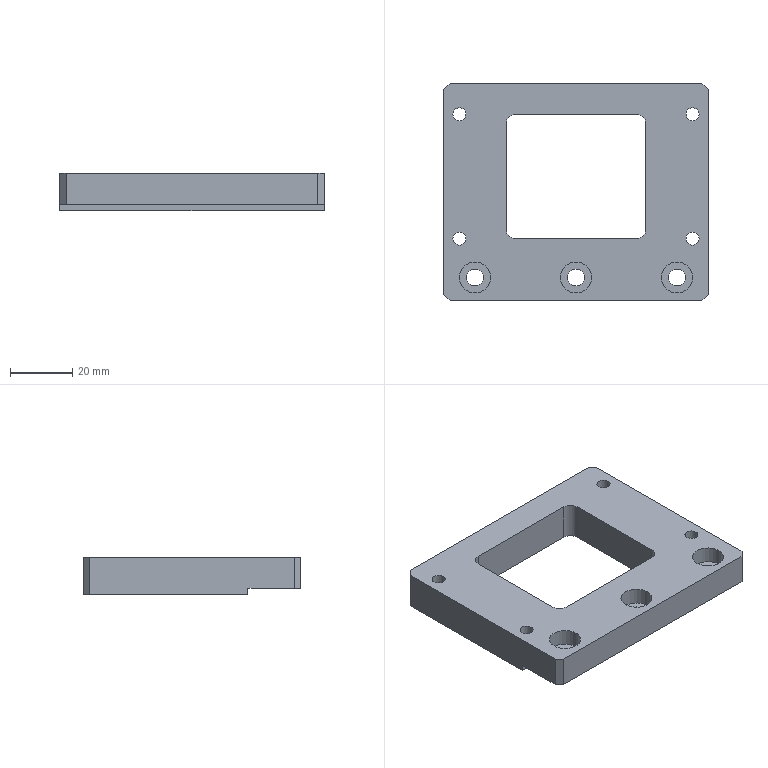CAM job | NX | 3-axis milling, drilling | part box 85 x 70 x 12 mm | stock box 90 x 75 x 15 mm
Tools:
number,name,description,diameter,corner_radius,flute_length,length,flutes
6,D6,平底铣刀-粗,6.0,0.0,25.0,75.0,2
9,D10,平底铣刀-粗,10.0,0.0,35.0,75.0,2
7,D6-J,平底铣刀-精,6.0,0.0,25.0,75.0,2
10,D10-J,平底铣刀-精,10.0,0.0,35.0,75.0,2
1,D80R0.8飞刀,圆鼻刀-粗,80.0,0.8,50.0,75.0,2
1,D80R0.8飞刀-J,圆鼻刀-精,80.0,0.8,50.0,75.0,2
2,D6倒角刀,倒角刀,6.0,0.0,3.0,25.0,2
22,M5X0.8,丝锥,4.2,0.0,35.0,50.0,2
17,ZT5.5,钻头,5.5,0.0,35.0,50.0,2
14,钻头4.2,Twist Drill 4.2 mm,4.2,0.0,41.0,41.738,2
Operations:
program,operation,operation_type,tool,method,geometry_group,spindle_rpm,surface_speed,feed_per_tooth,feed_cut,feed_plunge,cut_length_mm,path_length_mm,cut_time_min,machine_time_min
B,底壁铣飞面一刀开粗_COPY,VolumeBased25DMillingOperation,D80R0.8飞刀,分层开粗-切深K-步距G,W-B,2800.0,703.696,0.5357,3000.0,100.0,1159.164,2208.186,0.3864,0.4913
B,底壁铣飞面一刀精光_COPY,VolumeBased25DMillingOperation,D80R0.8飞刀-J,侧刃精光-切深K-步距G,W-B,4000.0,1005.28,0.125,1000.0,100.0,192.998,228.998,0.193,0.1966
B,底壁铣分层开粗-中_COPY,VolumeBased25DMillingOperation,D10,分层开粗-切深K-步距G,W-B,8000.0,251.327,0.3125,5000.0,100.0,1219.806,1546.104,0.244,0.2766
B,钻倒角_1,Operation,D6倒角刀,METHOD,W-B,8000.0,150.796,0.0625,1000.0,0.0,22.8,249.885,0.0228,0.0455
B,C0.3封闭铣廓倒角6X45L_COPY,PlanarMilling,D6倒角刀,爬面_倒角-切深0-步距G,W-B,7000.0,131.0,0.1071,1500.0,100.0,173.685,209.685,0.1158,0.1194
B,平面去毛刺6X45L_COPY,SurfaceContour,D6倒角刀,爬面_倒角-切深0-步距G,W-B,6500.0,122.519,0.1154,1500.0,100.0,650.68,1248.097,0.4338,0.4935
B,底壁铣精光底面-中_COPY,VolumeBased25DMillingOperation,D10-J,精光步距切深关,W-B,8000.0,251.32,0.0625,1000.0,100.0,397.288,423.887,0.3973,0.3999
B,底壁铣精光侧面-中-选底面_COPY,VolumeBased25DMillingOperation,D10-J,侧刃精光-切深K-步距G,W-B,8000.0,251.32,0.0625,1000.0,100.0,103.682,131.282,0.1037,0.1064
A,顶面,FaceMilling,D80R0.8飞刀,侧刃精光-切深K-步距G,W-A,4000.0,1005.31,0.125,1000.0,100.0,394.0,430.0,0.394,0.3976
A,外形粗_2,VolumeBased25DMillingOperation,D10,METHOD,W-A,8000.0,251.327,0.3125,5000.0,80.0,5736.6,5787.4,1.147,1.152
A,打点-深0.8,Operation,D6倒角刀,NONE,W-A,8000.0,150.796,0.0312,500.0,90.0,12.6,243.256,0.0252,0.0483
A,通孔-M5螺纹底孔,Operation,钻头4.2,NONE,W-A,3000.0,39.584,0.0583,350.0,90.0,81.047,360.126,0.2316,0.2595
A,沉头孔-钻孔0段,Operation,ZT5.5,NONE,W-A,1200.0,20.735,0.0625,150.0,90.0,43.957,194.945,0.293,0.3081
A,框开粗_1,VolumeBased25DMillingOperation,D10,METHOD,W-A,6000.0,188.0,0.25,4000.0,80.0,3360.723,3411.023,0.8402,0.8452
A,铣孔开粗D6_1,CylinderMilling,D6,NONE,W-A,8000.0,150.796,0.075,1200.0,100.0,476.699,676.399,0.3972,0.4172
A,铣孔精光D6_1,CylinderMilling,D6-J,精光步距切深关,W-A,8000.0,150.796,0.0312,500.0,100.0,100.196,301.396,0.2004,0.2205
A,清角D4,ZLevelMilling,D6-J,METHOD,W-A,6000.0,75.0,0.25,2500.0,80.0,1378.548,1568.653,0.5521,0.5711
A,框半精_1,VolumeBased25DMillingOperation,D6-J,METHOD,W-A,6000.0,113.0,0.0833,1000.0,100.0,151.042,213.042,0.151,0.1572
A,框精_1,VolumeBased25DMillingOperation,D6-J,METHOD,W-A,6000.0,113.0,0.0833,1000.0,100.0,150.842,213.442,0.1508,0.1571
A,仅选体,SurfaceContour,D6倒角刀,METHOD,W-A,8000.0,150.796,0.1875,3000.0,100.0,488.443,584.301,0.1628,0.1724
A,铣倒角_1,PlanarMilling,D6倒角刀,METHOD,W-A,8000.0,150.796,0.0312,500.0,100.0,72.081,391.094,0.1442,0.1761
A,铣倒角_2,PlanarMilling,D6倒角刀,NONE,W-A,8000.0,150.796,0.05,800.0,100.0,120.753,307.986,0.1509,0.1697
A,通孔-攻牙M5,Operation,M5X0.8,METHOD,W-A,500.0,6.597,0.0008,0.8,90.0,66.0,330.032,82.5,82.526
A,外形半精_2,VolumeBased25DMillingOperation,D10-J,METHOD,W-A,8000.0,251.327,0.0625,1000.0,100.0,341.688,405.288,0.3417,0.348